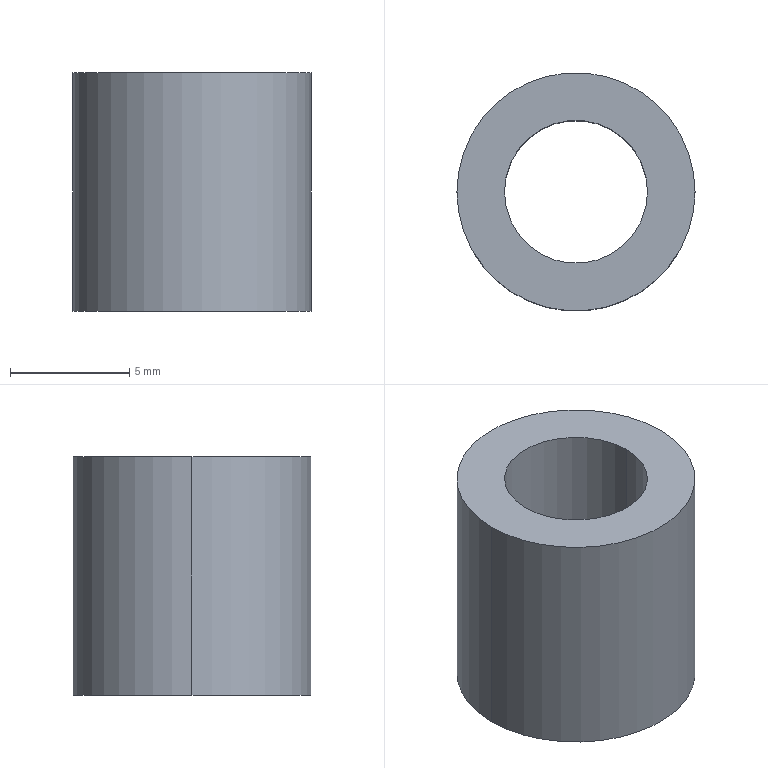Part | SolidWorks | features Extrusion 1 | 1 solid | 6 faces | box 9.99 x 9.99 x 10 mm | volume 501.085 mm3 | cylinder 4 | plane 2 | commonest cylinder face diameters 6 x2 9.99 x2
STEP:
#1=CARTESIAN_POINT('',(-3.,0.,10.));
#2=VERTEX_POINT('',#1);
#3=CARTESIAN_POINT('',(3.,0.,10.));
#4=VERTEX_POINT('',#3);
#5=CARTESIAN_POINT('',(0.,0.,10.));
#6=DIRECTION('',(0.,0.,1.));
#7=DIRECTION('',(1.,0.,0.));
#8=AXIS2_PLACEMENT_3D('',#5,#6,#7);
#9=CIRCLE('',#8,3.);
#10=EDGE_CURVE('',#2,#4,#9,.T.);
#11=ORIENTED_EDGE('',*,*,#10,.T.);
#12=CARTESIAN_POINT('',(3.,0.,0.));
#13=VERTEX_POINT('',#12);
#14=CARTESIAN_POINT('',(3.,0.,10.));
#15=DIRECTION('',(0.,0.,-1.));
#16=VECTOR('',#15,1000.);
#17=LINE('',#14,#16);
#18=EDGE_CURVE('',#4,#13,#17,.T.);
#19=ORIENTED_EDGE('',*,*,#18,.T.);
#20=CARTESIAN_POINT('',(-3.,0.,0.));
#21=VERTEX_POINT('',#20);
#22=CARTESIAN_POINT('',(0.,0.,0.));
#23=DIRECTION('',(0.,0.,1.));
#24=DIRECTION('',(1.,0.,0.));
#25=AXIS2_PLACEMENT_3D('',#22,#23,#24);
#26=CIRCLE('',#25,3.);
#27=EDGE_CURVE('',#21,#13,#26,.T.);
#28=ORIENTED_EDGE('',*,*,#27,.F.);
#29=CARTESIAN_POINT('',(-3.,0.,10.));
#30=DIRECTION('',(0.,0.,-1.));
#31=VECTOR('',#30,1000.);
#32=LINE('',#29,#31);
#33=EDGE_CURVE('',#2,#21,#32,.T.);
#34=ORIENTED_EDGE('',*,*,#33,.F.);
#35=EDGE_LOOP('',(#11,#19,#28,#34));
#36=FACE_OUTER_BOUND('',#35,.T.);
#37=CARTESIAN_POINT('',(0.,0.,10.));
#38=DIRECTION('',(0.,0.,-1.));
#39=DIRECTION('',(-1.,0.,0.));
#40=AXIS2_PLACEMENT_3D('',#37,#38,#39);
#41=CYLINDRICAL_SURFACE('',#40,3.);
#42=ADVANCED_FACE('',(#36),#41,.F.);
#43=CARTESIAN_POINT('',(4.995,0.,10.));
#44=VERTEX_POINT('',#43);
#45=CARTESIAN_POINT('',(-4.995,0.,10.));
#46=VERTEX_POINT('',#45);
#47=CARTESIAN_POINT('',(0.,0.,10.));
#48=DIRECTION('',(0.,0.,1.));
#49=DIRECTION('',(1.,0.,0.));
#50=AXIS2_PLACEMENT_3D('',#47,#48,#49);
#51=CIRCLE('',#50,4.995);
#52=EDGE_CURVE('',#44,#46,#51,.T.);
#53=ORIENTED_EDGE('',*,*,#52,.F.);
#54=CARTESIAN_POINT('',(4.995,0.,0.));
#55=VERTEX_POINT('',#54);
#56=CARTESIAN_POINT('',(4.995,0.,10.));
#57=DIRECTION('',(0.,0.,-1.));
#58=VECTOR('',#57,1000.);
#59=LINE('',#56,#58);
#60=EDGE_CURVE('',#44,#55,#59,.T.);
#61=ORIENTED_EDGE('',*,*,#60,.T.);
#62=CARTESIAN_POINT('',(-4.995,0.,0.));
#63=VERTEX_POINT('',#62);
#64=CARTESIAN_POINT('',(0.,0.,0.));
#65=DIRECTION('',(0.,0.,1.));
#66=DIRECTION('',(1.,0.,0.));
#67=AXIS2_PLACEMENT_3D('',#64,#65,#66);
#68=CIRCLE('',#67,4.995);
#69=EDGE_CURVE('',#55,#63,#68,.T.);
#70=ORIENTED_EDGE('',*,*,#69,.T.);
#71=CARTESIAN_POINT('',(-4.995,0.,10.));
#72=DIRECTION('',(0.,0.,-1.));
#73=VECTOR('',#72,1000.);
#74=LINE('',#71,#73);
#75=EDGE_CURVE('',#46,#63,#74,.T.);
#76=ORIENTED_EDGE('',*,*,#75,.F.);
#77=EDGE_LOOP('',(#53,#61,#70,#76));
#78=FACE_OUTER_BOUND('',#77,.T.);
#79=CARTESIAN_POINT('',(0.,0.,10.));
#80=DIRECTION('',(0.,0.,-1.));
#81=DIRECTION('',(-1.,0.,0.));
#82=AXIS2_PLACEMENT_3D('',#79,#80,#81);
#83=CYLINDRICAL_SURFACE('',#82,4.995);
#84=ADVANCED_FACE('',(#78),#83,.T.);
#85=CARTESIAN_POINT('',(0.,0.,10.));
#86=DIRECTION('',(0.,0.,1.));
#87=DIRECTION('',(1.,0.,0.));
#88=AXIS2_PLACEMENT_3D('',#85,#86,#87);
#89=CIRCLE('',#88,4.995);
#90=EDGE_CURVE('',#46,#44,#89,.T.);
#91=ORIENTED_EDGE('',*,*,#90,.T.);
#92=ORIENTED_EDGE('',*,*,#52,.T.);
#93=EDGE_LOOP('',(#91,#92));
#94=FACE_OUTER_BOUND('',#93,.T.);
#95=ORIENTED_EDGE('',*,*,#10,.F.);
#96=CARTESIAN_POINT('',(0.,0.,10.));
#97=DIRECTION('',(0.,0.,1.));
#98=DIRECTION('',(1.,0.,0.));
#99=AXIS2_PLACEMENT_3D('',#96,#97,#98);
#100=CIRCLE('',#99,3.);
#101=EDGE_CURVE('',#4,#2,#100,.T.);
#102=ORIENTED_EDGE('',*,*,#101,.F.);
#103=EDGE_LOOP('',(#95,#102));
#104=FACE_BOUND('',#103,.T.);
#105=CARTESIAN_POINT('',(0.,0.,10.));
#106=DIRECTION('',(0.,0.,1.));
#107=DIRECTION('',(1.,0.,0.));
#108=AXIS2_PLACEMENT_3D('',#105,#106,#107);
#109=PLANE('',#108);
#110=ADVANCED_FACE('',(#94,#104),#109,.T.);
#111=CARTESIAN_POINT('',(0.,0.,0.));
#112=DIRECTION('',(0.,0.,1.));
#113=DIRECTION('',(1.,0.,0.));
#114=AXIS2_PLACEMENT_3D('',#111,#112,#113);
#115=CIRCLE('',#114,4.995);
#116=EDGE_CURVE('',#63,#55,#115,.T.);
#117=ORIENTED_EDGE('',*,*,#116,.F.);
#118=ORIENTED_EDGE('',*,*,#69,.F.);
#119=EDGE_LOOP('',(#117,#118));
#120=FACE_OUTER_BOUND('',#119,.T.);
#121=ORIENTED_EDGE('',*,*,#27,.T.);
#122=CARTESIAN_POINT('',(0.,0.,0.));
#123=DIRECTION('',(0.,0.,1.));
#124=DIRECTION('',(1.,0.,0.));
#125=AXIS2_PLACEMENT_3D('',#122,#123,#124);
#126=CIRCLE('',#125,3.);
#127=EDGE_CURVE('',#13,#21,#126,.T.);
#128=ORIENTED_EDGE('',*,*,#127,.T.);
#129=EDGE_LOOP('',(#121,#128));
#130=FACE_BOUND('',#129,.T.);
#131=CARTESIAN_POINT('',(0.,0.,0.));
#132=DIRECTION('',(0.,0.,1.));
#133=DIRECTION('',(1.,0.,0.));
#134=AXIS2_PLACEMENT_3D('',#131,#132,#133);
#135=PLANE('',#134);
#136=ADVANCED_FACE('',(#120,#130),#135,.F.);
#137=ORIENTED_EDGE('',*,*,#60,.F.);
#138=ORIENTED_EDGE('',*,*,#90,.F.);
#139=ORIENTED_EDGE('',*,*,#75,.T.);
#140=ORIENTED_EDGE('',*,*,#116,.T.);
#141=EDGE_LOOP('',(#137,#138,#139,#140));
#142=FACE_OUTER_BOUND('',#141,.T.);
#143=CARTESIAN_POINT('',(0.,0.,10.));
#144=DIRECTION('',(0.,0.,-1.));
#145=DIRECTION('',(-1.,0.,0.));
#146=AXIS2_PLACEMENT_3D('',#143,#144,#145);
#147=CYLINDRICAL_SURFACE('',#146,4.995);
#148=ADVANCED_FACE('',(#142),#147,.T.);
#149=ORIENTED_EDGE('',*,*,#18,.F.);
#150=ORIENTED_EDGE('',*,*,#101,.T.);
#151=ORIENTED_EDGE('',*,*,#33,.T.);
#152=ORIENTED_EDGE('',*,*,#127,.F.);
#153=EDGE_LOOP('',(#149,#150,#151,#152));
#154=FACE_OUTER_BOUND('',#153,.T.);
#155=CARTESIAN_POINT('',(0.,0.,10.));
#156=DIRECTION('',(0.,0.,-1.));
#157=DIRECTION('',(-1.,0.,0.));
#158=AXIS2_PLACEMENT_3D('',#155,#156,#157);
#159=CYLINDRICAL_SURFACE('',#158,3.);
#160=ADVANCED_FACE('',(#154),#159,.F.);
#161=CLOSED_SHELL('',(#42,#84,#110,#136,#148,#160));
#162=MANIFOLD_SOLID_BREP('',#161);
#163=CARTESIAN_POINT('',(0.,0.,0.));
#164=DIRECTION('',(0.,0.,1.));
#165=DIRECTION('',(1.,0.,0.));
#166=AXIS2_PLACEMENT_3D('',#163,#164,#165);
#167=(LENGTH_UNIT()NAMED_UNIT(*)SI_UNIT(.MILLI.,.METRE.));
#168=UNCERTAINTY_MEASURE_WITH_UNIT(LENGTH_MEASURE(0.00001),#167,'','');
#169=(NAMED_UNIT(*)PLANE_ANGLE_UNIT()SI_UNIT($,.RADIAN.));
#170=(NAMED_UNIT(*)SI_UNIT($,.STERADIAN.)SOLID_ANGLE_UNIT());
#171=(GEOMETRIC_REPRESENTATION_CONTEXT(3)GLOBAL_UNCERTAINTY_ASSIGNED_CONTEXT((#168))GLOBAL_UNIT_ASSIGNED_CONTEXT((#167,#169,#170))REPRESENTATION_CONTEXT('',''));
#172=ADVANCED_BREP_SHAPE_REPRESENTATION('',(#162,#166),#171);